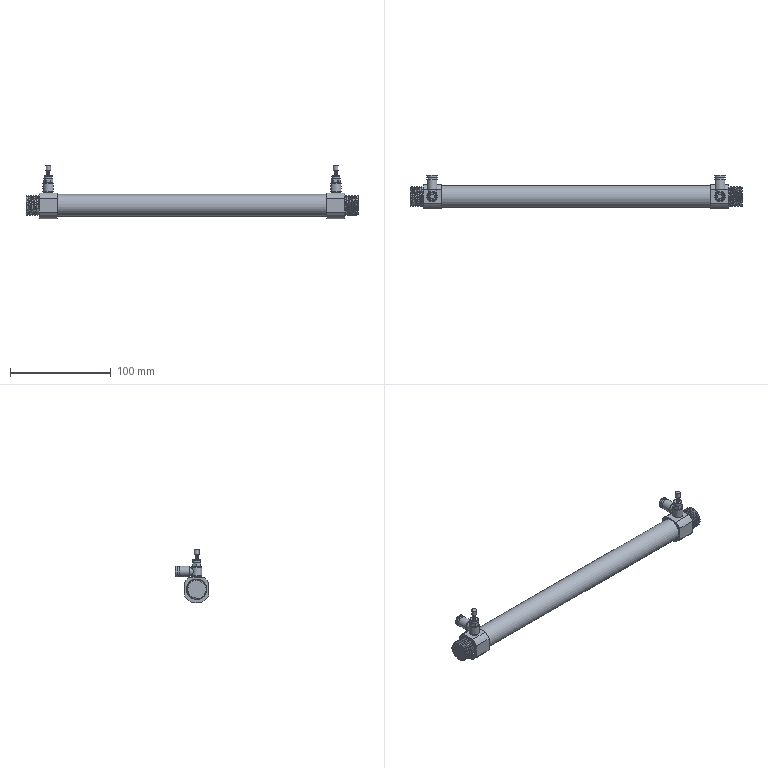Part | STEP file | Tube feed_id810_x_t | 1 solid | 195 faces | box 330 x 33.15 x 53.75 mm | volume 129080 mm3 | plane 136 | cylinder 33 | spline 12 | torus 12 | cone 2 | commonest cylinder face diameters 8 x6 27.5 x6 10.3 x4 2.5 x2 3 x2 5 x2